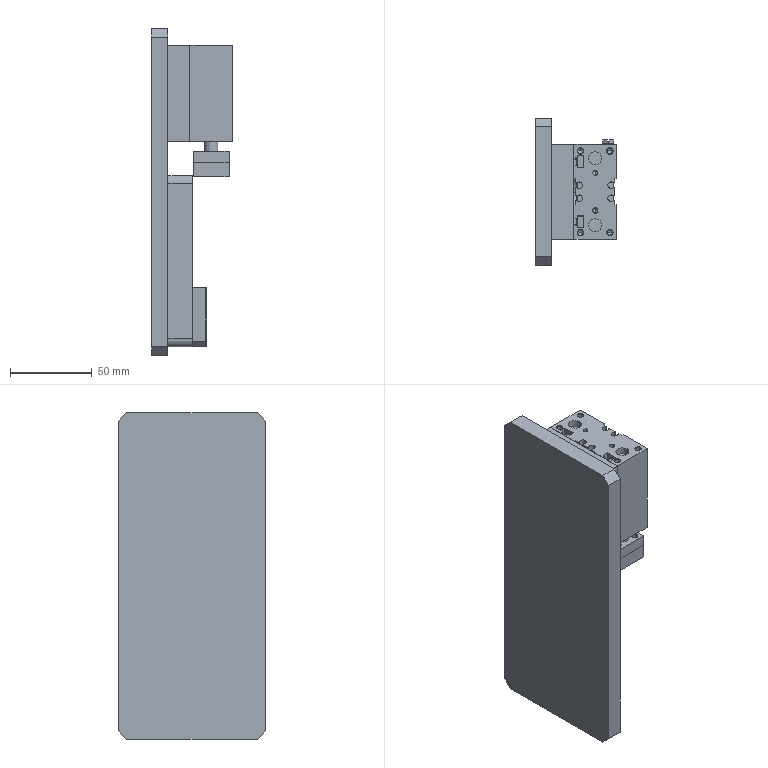Part | SolidWorks | 9 solids | 425 faces | box 49.5 x 90 x 200 mm | volume 386191 mm3 | plane 172 | cylinder 137 | cone 104 | spline 12 | commonest cylinder face diameters 0.28 x18 3 x18 3.242 x16 4.134 x16 8 x16 4.3 x8